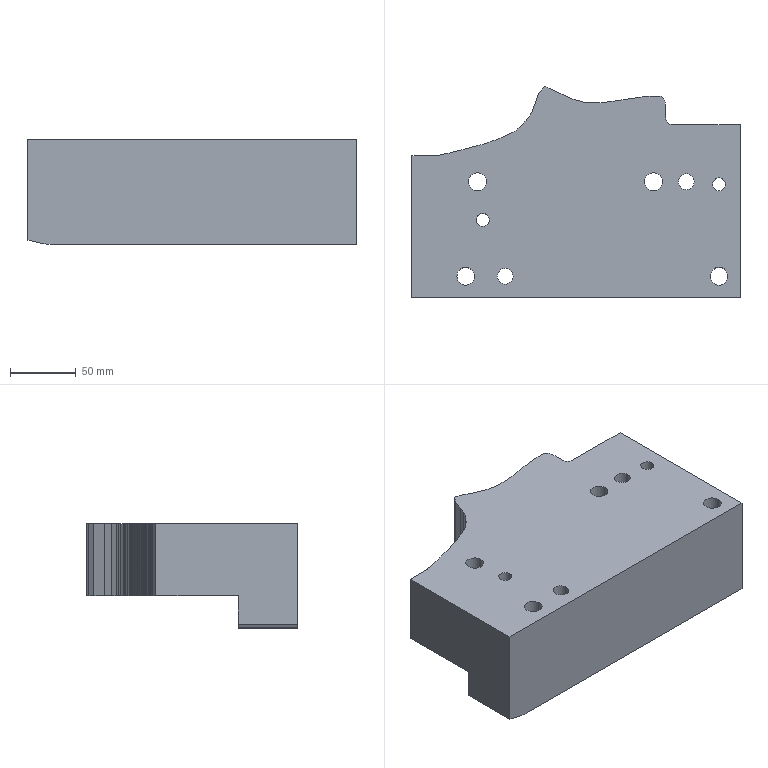Part | STEP file | lll_id642_x_t | 1 solid | 101 faces | box 250 x 160.491 x 80 mm | volume 2027963 mm3 | plane 72 | cylinder 23 | cone 6 | commonest cylinder face diameters 8.506 x5 13.509 x4 20.007 x4 10 x2 11 x2 12 x2